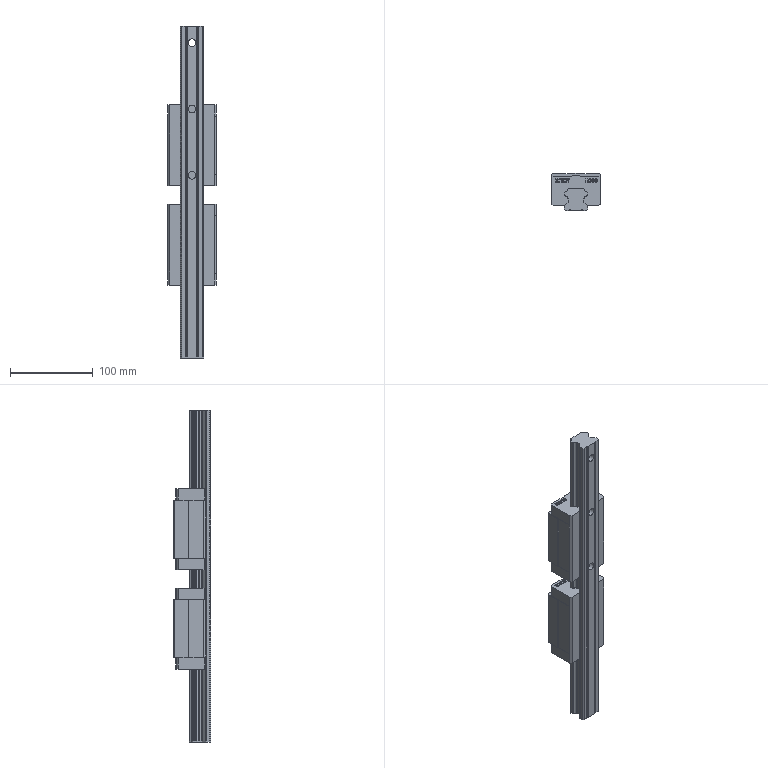Part | SolidWorks | features LocalLPattern 1, ReferencePattern 1 | 3 solids | 847 faces | box 60 x 45 x 400 mm | volume 578524 mm3 | plane 637 | spline 120 | cylinder 90 | commonest cylinder face diameters 1.2 x36 8 x16 1.6 x14 5.66 x12 9 x6 14 x6